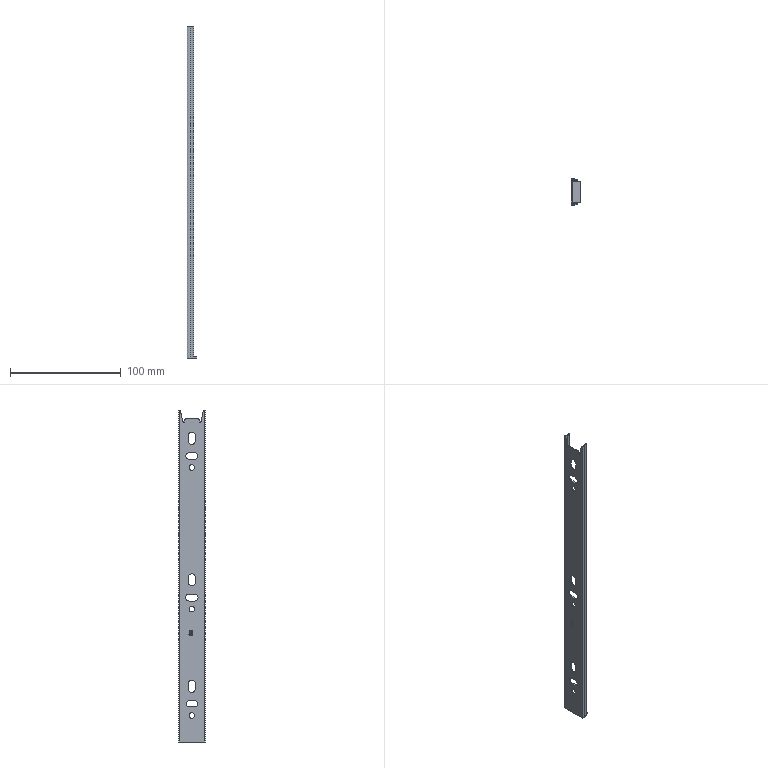Part | STEP file | slide rail 300-3 | 1 solid | 122 faces | box 9.001 x 23.751 x 300 mm | volume 9128 mm3 | plane 52 | cylinder 39 | spline 31 | commonest cylinder face diameters 3 x6 6.367 x4 0.4 x3 5 x3 1 x2 1.12 x2